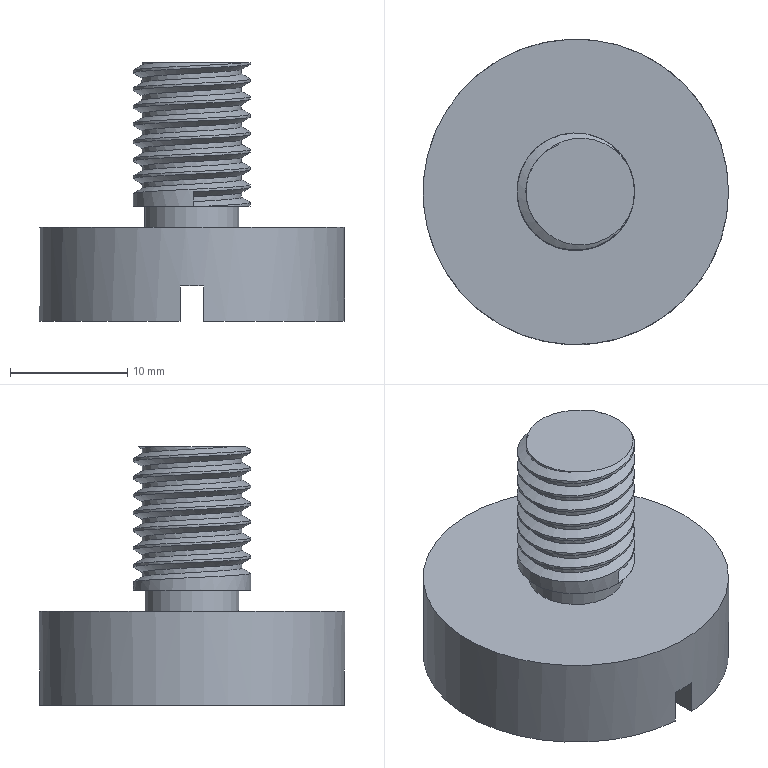Part | NX | features CYLINDER 2, DATUM_CSYS 2, EXTRUDE 1, RECT_GROOVE 1, SKETCH 1, THREADS 1 | 2 solids | 16 faces | box 26 x 26 x 22 mm | volume 4995 mm3 | plane 10 | cylinder 4 | spline 2 | commonest cylinder face diameters 8 x1 8.5 x1 10 x1 26 x1